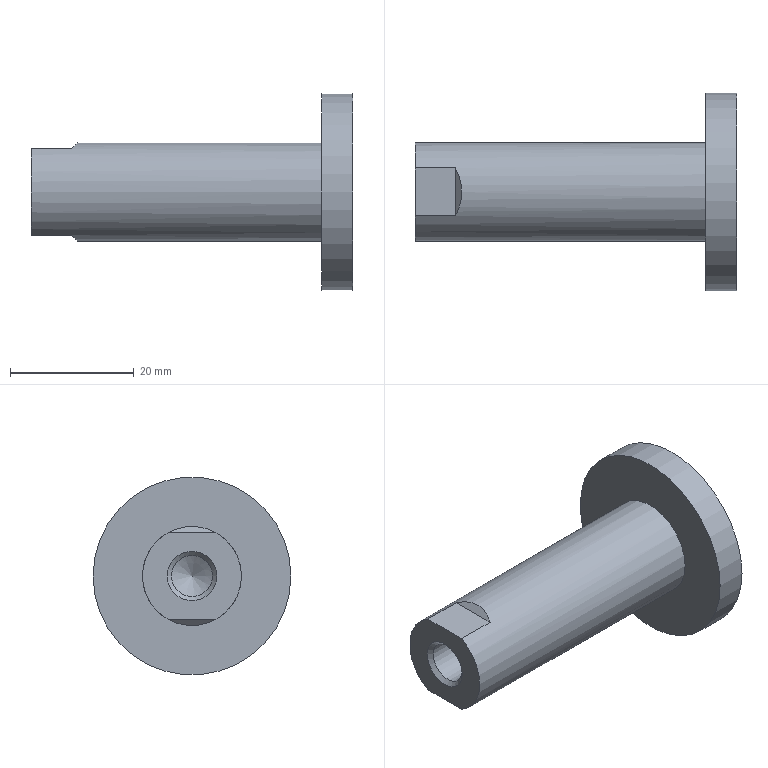Part | NX | 1 solid | 12 faces | box 52 x 32 x 32 mm | volume 12921 mm3 | plane 7 | cylinder 3 | cone 2 | commonest cylinder face diameters 6.647 x1 16 x1 32 x1
STEP:
#1=CARTESIAN_POINT('',(7.919,0.,0.));
#2=VERTEX_POINT('',#1);
#3=VERTEX_LOOP('',#2);
#4=FACE_BOUND('',#3,.T.);
#5=CARTESIAN_POINT('',(6.,-3.324,0.));
#6=VERTEX_POINT('',#5);
#7=CARTESIAN_POINT('',(6.,0.,0.));
#8=DIRECTION('',(-1.,0.,0.));
#9=DIRECTION('',(0.,-1.,0.));
#10=AXIS2_PLACEMENT_3D('',#7,#8,#9);
#11=CIRCLE('',#10,3.324);
#12=EDGE_CURVE('',#6,#6,#11,.T.);
#13=ORIENTED_EDGE('',*,*,#12,.T.);
#14=EDGE_LOOP('',(#13));
#15=FACE_BOUND('',#14,.T.);
#16=CARTESIAN_POINT('',(6.,0.,0.));
#17=DIRECTION('',(-1.,0.,0.));
#18=DIRECTION('',(0.,-1.,0.));
#19=AXIS2_PLACEMENT_3D('',#16,#17,#18);
#20=CONICAL_SURFACE('',#19,3.324,1.047);
#21=ADVANCED_FACE('',(#4,#15),#20,.F.);
#22=ORIENTED_EDGE('',*,*,#12,.F.);
#23=EDGE_LOOP('',(#22));
#24=FACE_BOUND('',#23,.T.);
#25=CARTESIAN_POINT('',(-6.324,-3.323,0.));
#26=VERTEX_POINT('',#25);
#27=CARTESIAN_POINT('',(-6.324,0.,0.));
#28=DIRECTION('',(-1.,0.,0.));
#29=DIRECTION('',(0.,-1.,0.));
#30=AXIS2_PLACEMENT_3D('',#27,#28,#29);
#31=CIRCLE('',#30,3.324);
#32=EDGE_CURVE('',#26,#26,#31,.T.);
#33=ORIENTED_EDGE('',*,*,#32,.T.);
#34=EDGE_LOOP('',(#33));
#35=FACE_BOUND('',#34,.T.);
#36=CARTESIAN_POINT('',(45.,0.,0.));
#37=DIRECTION('',(-1.,0.,0.));
#38=DIRECTION('',(0.,-1.,0.));
#39=AXIS2_PLACEMENT_3D('',#36,#37,#38);
#40=CYLINDRICAL_SURFACE('',#39,3.324);
#41=ADVANCED_FACE('',(#24,#35),#40,.F.);
#42=ORIENTED_EDGE('',*,*,#32,.F.);
#43=EDGE_LOOP('',(#42));
#44=FACE_BOUND('',#43,.T.);
#45=CARTESIAN_POINT('',(-7.,-4.,0.));
#46=VERTEX_POINT('',#45);
#47=CARTESIAN_POINT('',(-7.,0.,0.));
#48=DIRECTION('',(-1.,0.,0.));
#49=DIRECTION('',(0.,-1.,0.));
#50=AXIS2_PLACEMENT_3D('',#47,#48,#49);
#51=CIRCLE('',#50,4.);
#52=EDGE_CURVE('',#46,#46,#51,.T.);
#53=ORIENTED_EDGE('',*,*,#52,.T.);
#54=EDGE_LOOP('',(#53));
#55=FACE_BOUND('',#54,.T.);
#56=CARTESIAN_POINT('',(-7.,0.,0.));
#57=DIRECTION('',(-1.,0.,0.));
#58=DIRECTION('',(0.,-1.,0.));
#59=AXIS2_PLACEMENT_3D('',#56,#57,#58);
#60=CONICAL_SURFACE('',#59,4.,0.7854);
#61=ADVANCED_FACE('',(#44,#55),#60,.F.);
#62=ORIENTED_EDGE('',*,*,#52,.F.);
#63=EDGE_LOOP('',(#62));
#64=FACE_BOUND('',#63,.T.);
#65=CARTESIAN_POINT('',(-7.,3.873,7.));
#66=VERTEX_POINT('',#65);
#67=CARTESIAN_POINT('',(-7.,3.873,-7.));
#68=VERTEX_POINT('',#67);
#69=CARTESIAN_POINT('',(-7.,0.,0.));
#70=DIRECTION('',(-1.,0.,0.));
#71=DIRECTION('',(0.,-1.,0.));
#72=AXIS2_PLACEMENT_3D('',#69,#70,#71);
#73=CIRCLE('',#72,8.);
#74=EDGE_CURVE('',#66,#68,#73,.T.);
#75=ORIENTED_EDGE('',*,*,#74,.T.);
#76=CARTESIAN_POINT('',(-7.,-3.873,-7.));
#77=VERTEX_POINT('',#76);
#78=CARTESIAN_POINT('',(-7.,-16.,-7.));
#79=DIRECTION('',(0.,1.,0.));
#80=VECTOR('',#79,1000.);
#81=LINE('',#78,#80);
#82=EDGE_CURVE('',#77,#68,#81,.T.);
#83=ORIENTED_EDGE('',*,*,#82,.F.);
#84=CARTESIAN_POINT('',(-7.,-3.873,7.));
#85=VERTEX_POINT('',#84);
#86=CARTESIAN_POINT('',(-7.,0.,0.));
#87=DIRECTION('',(-1.,0.,0.));
#88=DIRECTION('',(0.,-1.,0.));
#89=AXIS2_PLACEMENT_3D('',#86,#87,#88);
#90=CIRCLE('',#89,8.);
#91=EDGE_CURVE('',#77,#85,#90,.T.);
#92=ORIENTED_EDGE('',*,*,#91,.T.);
#93=CARTESIAN_POINT('',(-7.,-16.,7.));
#94=DIRECTION('',(0.,1.,0.));
#95=VECTOR('',#94,1000.);
#96=LINE('',#93,#95);
#97=EDGE_CURVE('',#85,#66,#96,.T.);
#98=ORIENTED_EDGE('',*,*,#97,.T.);
#99=EDGE_LOOP('',(#75,#83,#92,#98));
#100=FACE_BOUND('',#99,.T.);
#101=CARTESIAN_POINT('',(-7.,4.,0.));
#102=DIRECTION('',(1.,0.,0.));
#103=DIRECTION('',(0.,1.,0.));
#104=AXIS2_PLACEMENT_3D('',#101,#102,#103);
#105=PLANE('',#104);
#106=ADVANCED_FACE('',(#64,#100),#105,.F.);
#107=CARTESIAN_POINT('',(-0.5,-3.873,-7.));
#108=VERTEX_POINT('',#107);
#109=CARTESIAN_POINT('',(-0.5,3.873,-7.));
#110=VERTEX_POINT('',#109);
#111=CARTESIAN_POINT('',(-7.5,0.,0.));
#112=DIRECTION('',(0.7071,0.,0.7071));
#113=DIRECTION('',(-0.7071,0.,0.7071));
#114=AXIS2_PLACEMENT_3D('',#111,#112,#113);
#115=ELLIPSE('',#114,11.314,8.);
#116=EDGE_CURVE('',#108,#110,#115,.T.);
#117=ORIENTED_EDGE('',*,*,#116,.T.);
#118=CARTESIAN_POINT('',(45.,3.873,-7.));
#119=DIRECTION('',(-1.,0.,0.));
#120=VECTOR('',#119,1000.);
#121=LINE('',#118,#120);
#122=EDGE_CURVE('',#110,#68,#121,.T.);
#123=ORIENTED_EDGE('',*,*,#122,.T.);
#124=ORIENTED_EDGE('',*,*,#74,.F.);
#125=CARTESIAN_POINT('',(-0.5,3.873,7.));
#126=VERTEX_POINT('',#125);
#127=CARTESIAN_POINT('',(45.,3.873,7.));
#128=DIRECTION('',(-1.,0.,0.));
#129=VECTOR('',#128,1000.);
#130=LINE('',#127,#129);
#131=EDGE_CURVE('',#66,#126,#130,.F.);
#132=ORIENTED_EDGE('',*,*,#131,.T.);
#133=CARTESIAN_POINT('',(-0.5,-3.873,7.));
#134=VERTEX_POINT('',#133);
#135=CARTESIAN_POINT('',(-7.5,0.,0.));
#136=DIRECTION('',(0.7071,0.,-0.7071));
#137=DIRECTION('',(-0.7071,0.,-0.7071));
#138=AXIS2_PLACEMENT_3D('',#135,#136,#137);
#139=ELLIPSE('',#138,11.314,8.);
#140=EDGE_CURVE('',#126,#134,#139,.T.);
#141=ORIENTED_EDGE('',*,*,#140,.T.);
#142=CARTESIAN_POINT('',(45.,-3.873,7.));
#143=DIRECTION('',(-1.,0.,0.));
#144=VECTOR('',#143,1000.);
#145=LINE('',#142,#144);
#146=EDGE_CURVE('',#134,#85,#145,.T.);
#147=ORIENTED_EDGE('',*,*,#146,.T.);
#148=ORIENTED_EDGE('',*,*,#91,.F.);
#149=CARTESIAN_POINT('',(45.,-3.873,-7.));
#150=DIRECTION('',(-1.,0.,0.));
#151=VECTOR('',#150,1000.);
#152=LINE('',#149,#151);
#153=EDGE_CURVE('',#77,#108,#152,.F.);
#154=ORIENTED_EDGE('',*,*,#153,.T.);
#155=EDGE_LOOP('',(#117,#123,#124,#132,#141,#147,#148,#154));
#156=FACE_BOUND('',#155,.T.);
#157=CARTESIAN_POINT('',(40.,-8.,0.));
#158=VERTEX_POINT('',#157);
#159=CARTESIAN_POINT('',(40.,0.,0.));
#160=DIRECTION('',(-1.,0.,0.));
#161=DIRECTION('',(0.,-1.,0.));
#162=AXIS2_PLACEMENT_3D('',#159,#160,#161);
#163=CIRCLE('',#162,8.);
#164=EDGE_CURVE('',#158,#158,#163,.T.);
#165=ORIENTED_EDGE('',*,*,#164,.T.);
#166=EDGE_LOOP('',(#165));
#167=FACE_BOUND('',#166,.T.);
#168=CARTESIAN_POINT('',(45.,0.,0.));
#169=DIRECTION('',(-1.,0.,0.));
#170=DIRECTION('',(0.,-1.,0.));
#171=AXIS2_PLACEMENT_3D('',#168,#169,#170);
#172=CYLINDRICAL_SURFACE('',#171,8.);
#173=ADVANCED_FACE('',(#156,#167),#172,.T.);
#174=ORIENTED_EDGE('',*,*,#164,.F.);
#175=EDGE_LOOP('',(#174));
#176=FACE_BOUND('',#175,.T.);
#177=CARTESIAN_POINT('',(40.,-16.,0.));
#178=VERTEX_POINT('',#177);
#179=CARTESIAN_POINT('',(40.,0.,0.));
#180=DIRECTION('',(-1.,0.,0.));
#181=DIRECTION('',(0.,-1.,0.));
#182=AXIS2_PLACEMENT_3D('',#179,#180,#181);
#183=CIRCLE('',#182,16.);
#184=EDGE_CURVE('',#178,#178,#183,.T.);
#185=ORIENTED_EDGE('',*,*,#184,.T.);
#186=EDGE_LOOP('',(#185));
#187=FACE_BOUND('',#186,.T.);
#188=CARTESIAN_POINT('',(40.,8.,0.));
#189=DIRECTION('',(1.,0.,0.));
#190=DIRECTION('',(0.,1.,0.));
#191=AXIS2_PLACEMENT_3D('',#188,#189,#190);
#192=PLANE('',#191);
#193=ADVANCED_FACE('',(#176,#187),#192,.F.);
#194=ORIENTED_EDGE('',*,*,#184,.F.);
#195=EDGE_LOOP('',(#194));
#196=FACE_BOUND('',#195,.T.);
#197=CARTESIAN_POINT('',(45.,-16.,0.));
#198=VERTEX_POINT('',#197);
#199=CARTESIAN_POINT('',(45.,0.,0.));
#200=DIRECTION('',(-1.,0.,0.));
#201=DIRECTION('',(0.,-1.,0.));
#202=AXIS2_PLACEMENT_3D('',#199,#200,#201);
#203=CIRCLE('',#202,16.);
#204=EDGE_CURVE('',#198,#198,#203,.T.);
#205=ORIENTED_EDGE('',*,*,#204,.T.);
#206=EDGE_LOOP('',(#205));
#207=FACE_BOUND('',#206,.T.);
#208=CARTESIAN_POINT('',(45.,0.,0.));
#209=DIRECTION('',(-1.,0.,0.));
#210=DIRECTION('',(0.,-1.,0.));
#211=AXIS2_PLACEMENT_3D('',#208,#209,#210);
#212=CYLINDRICAL_SURFACE('',#211,16.);
#213=ADVANCED_FACE('',(#196,#207),#212,.T.);
#214=ORIENTED_EDGE('',*,*,#204,.F.);
#215=EDGE_LOOP('',(#214));
#216=FACE_BOUND('',#215,.T.);
#217=CARTESIAN_POINT('',(45.,16.,0.));
#218=DIRECTION('',(-1.,0.,0.));
#219=DIRECTION('',(0.,-1.,0.));
#220=AXIS2_PLACEMENT_3D('',#217,#218,#219);
#221=PLANE('',#220);
#222=ADVANCED_FACE('',(#216),#221,.F.);
#223=CARTESIAN_POINT('',(-0.5,-16.,7.));
#224=DIRECTION('',(0.,1.,0.));
#225=VECTOR('',#224,1000.);
#226=LINE('',#223,#225);
#227=EDGE_CURVE('',#134,#126,#226,.T.);
#228=ORIENTED_EDGE('',*,*,#227,.F.);
#229=ORIENTED_EDGE('',*,*,#140,.F.);
#230=EDGE_LOOP('',(#228,#229));
#231=FACE_BOUND('',#230,.T.);
#232=CARTESIAN_POINT('',(4.5,-16.,12.));
#233=DIRECTION('',(0.7071,0.,-0.7071));
#234=DIRECTION('',(-0.7071,0.,-0.7071));
#235=AXIS2_PLACEMENT_3D('',#232,#233,#234);
#236=PLANE('',#235);
#237=ADVANCED_FACE('',(#231),#236,.F.);
#238=ORIENTED_EDGE('',*,*,#227,.T.);
#239=ORIENTED_EDGE('',*,*,#131,.F.);
#240=ORIENTED_EDGE('',*,*,#97,.F.);
#241=ORIENTED_EDGE('',*,*,#146,.F.);
#242=EDGE_LOOP('',(#238,#239,#240,#241));
#243=FACE_BOUND('',#242,.T.);
#244=CARTESIAN_POINT('',(-0.5,-16.,7.));
#245=DIRECTION('',(0.,0.,-1.));
#246=DIRECTION('',(-1.,0.,0.));
#247=AXIS2_PLACEMENT_3D('',#244,#245,#246);
#248=PLANE('',#247);
#249=ADVANCED_FACE('',(#243),#248,.F.);
#250=CARTESIAN_POINT('',(-0.5,-16.,-7.));
#251=DIRECTION('',(0.,1.,0.));
#252=VECTOR('',#251,1000.);
#253=LINE('',#250,#252);
#254=EDGE_CURVE('',#108,#110,#253,.T.);
#255=ORIENTED_EDGE('',*,*,#254,.T.);
#256=ORIENTED_EDGE('',*,*,#116,.F.);
#257=EDGE_LOOP('',(#255,#256));
#258=FACE_BOUND('',#257,.T.);
#259=CARTESIAN_POINT('',(-0.5,-16.,-7.));
#260=DIRECTION('',(0.7071,0.,0.7071));
#261=DIRECTION('',(0.7071,0.,-0.7071));
#262=AXIS2_PLACEMENT_3D('',#259,#260,#261);
#263=PLANE('',#262);
#264=ADVANCED_FACE('',(#258),#263,.F.);
#265=ORIENTED_EDGE('',*,*,#254,.F.);
#266=ORIENTED_EDGE('',*,*,#153,.F.);
#267=ORIENTED_EDGE('',*,*,#82,.T.);
#268=ORIENTED_EDGE('',*,*,#122,.F.);
#269=EDGE_LOOP('',(#265,#266,#267,#268));
#270=FACE_BOUND('',#269,.T.);
#271=CARTESIAN_POINT('',(-7.,-16.,-7.));
#272=DIRECTION('',(0.,0.,1.));
#273=DIRECTION('',(1.,0.,0.));
#274=AXIS2_PLACEMENT_3D('',#271,#272,#273);
#275=PLANE('',#274);
#276=ADVANCED_FACE('',(#270),#275,.F.);
#277=CLOSED_SHELL('',(#21,#41,#61,#106,#173,#193,#213,#222,#237,#249,#264,#276));
#278=MANIFOLD_SOLID_BREP('',#277);
#279=(LENGTH_UNIT()NAMED_UNIT(*)SI_UNIT(.MILLI.,.METRE.));
#280=UNCERTAINTY_MEASURE_WITH_UNIT(LENGTH_MEASURE(0.00001),#279,'','');
#281=(NAMED_UNIT(*)PLANE_ANGLE_UNIT()SI_UNIT($,.RADIAN.));
#282=(NAMED_UNIT(*)SI_UNIT($,.STERADIAN.)SOLID_ANGLE_UNIT());
#283=(GEOMETRIC_REPRESENTATION_CONTEXT(3)GLOBAL_UNCERTAINTY_ASSIGNED_CONTEXT((#280))GLOBAL_UNIT_ASSIGNED_CONTEXT((#279,#281,#282))REPRESENTATION_CONTEXT('',''));
#284=ADVANCED_BREP_SHAPE_REPRESENTATION('',(#278),#283);